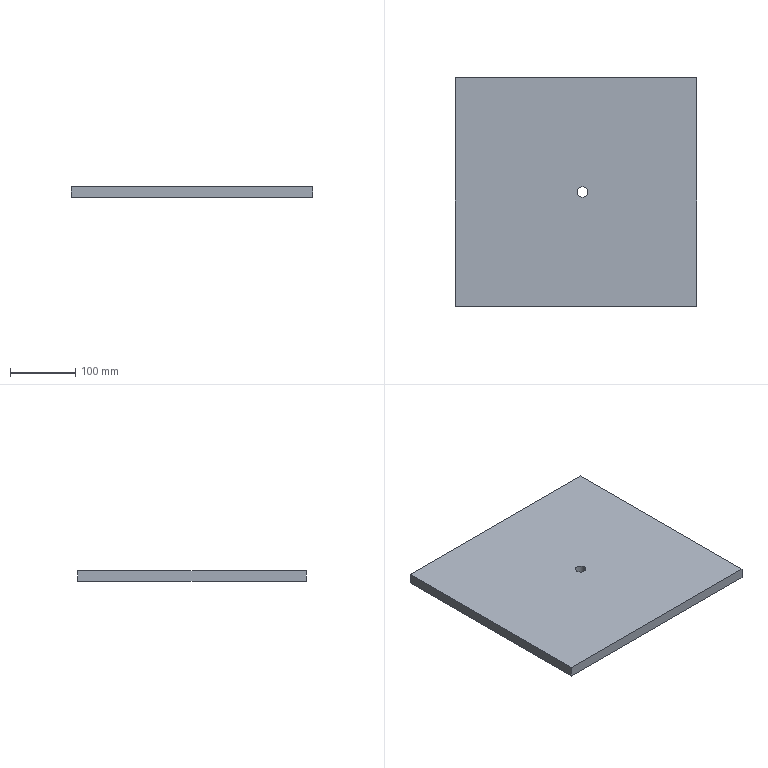Part | SolidWorks | features BaseBody 1 | 1 solid | 8 faces | box 370 x 350 x 16 mm | volume 2068783 mm3 | plane 6 | cylinder 2 | commonest cylinder face diameters 16 x2
STEP:
#1=CARTESIAN_POINT('',(-142.453,1729.544,-1224.));
#2=VERTEX_POINT('',#1);
#3=CARTESIAN_POINT('',(-126.453,1729.544,-1224.));
#4=VERTEX_POINT('',#3);
#5=CARTESIAN_POINT('',(-134.453,1729.544,-1224.));
#6=DIRECTION('',(0.,0.,1.));
#7=DIRECTION('',(1.,0.,0.));
#8=AXIS2_PLACEMENT_3D('',#5,#6,#7);
#9=CIRCLE('',#8,8.);
#10=EDGE_CURVE('',#2,#4,#9,.T.);
#11=ORIENTED_EDGE('',*,*,#10,.F.);
#12=CARTESIAN_POINT('',(-142.453,1729.544,-1208.));
#13=VERTEX_POINT('',#12);
#14=CARTESIAN_POINT('',(-142.453,1729.544,-1246.627));
#15=DIRECTION('',(0.,0.,1.));
#16=VECTOR('',#15,1000.);
#17=LINE('',#14,#16);
#18=EDGE_CURVE('',#2,#13,#17,.T.);
#19=ORIENTED_EDGE('',*,*,#18,.T.);
#20=CARTESIAN_POINT('',(-126.453,1729.544,-1208.));
#21=VERTEX_POINT('',#20);
#22=CARTESIAN_POINT('',(-134.453,1729.544,-1208.));
#23=DIRECTION('',(0.,0.,-1.));
#24=DIRECTION('',(1.,0.,0.));
#25=AXIS2_PLACEMENT_3D('',#22,#23,#24);
#26=CIRCLE('',#25,8.);
#27=EDGE_CURVE('',#21,#13,#26,.T.);
#28=ORIENTED_EDGE('',*,*,#27,.F.);
#29=CARTESIAN_POINT('',(-126.453,1729.544,-1246.627));
#30=DIRECTION('',(0.,0.,1.));
#31=VECTOR('',#30,1000.);
#32=LINE('',#29,#31);
#33=EDGE_CURVE('',#4,#21,#32,.T.);
#34=ORIENTED_EDGE('',*,*,#33,.F.);
#35=EDGE_LOOP('',(#11,#19,#28,#34));
#36=FACE_OUTER_BOUND('',#35,.T.);
#37=CARTESIAN_POINT('',(-134.453,1729.544,-1246.627));
#38=DIRECTION('',(0.,0.,1.));
#39=DIRECTION('',(1.,0.,0.));
#40=AXIS2_PLACEMENT_3D('',#37,#38,#39);
#41=CYLINDRICAL_SURFACE('',#40,8.);
#42=ADVANCED_FACE('',(#36),#41,.F.);
#43=ORIENTED_EDGE('',*,*,#27,.T.);
#44=CARTESIAN_POINT('',(-134.453,1729.544,-1208.));
#45=DIRECTION('',(0.,0.,-1.));
#46=DIRECTION('',(1.,0.,0.));
#47=AXIS2_PLACEMENT_3D('',#44,#45,#46);
#48=CIRCLE('',#47,8.);
#49=EDGE_CURVE('',#13,#21,#48,.T.);
#50=ORIENTED_EDGE('',*,*,#49,.T.);
#51=EDGE_LOOP('',(#43,#50));
#52=FACE_BOUND('',#51,.T.);
#53=CARTESIAN_POINT('',(40.547,1554.544,-1208.));
#54=VERTEX_POINT('',#53);
#55=CARTESIAN_POINT('',(40.547,1904.544,-1208.));
#56=VERTEX_POINT('',#55);
#57=CARTESIAN_POINT('',(40.547,1904.544,-1208.));
#58=DIRECTION('',(0.,1.,0.));
#59=VECTOR('',#58,1000.);
#60=LINE('',#57,#59);
#61=EDGE_CURVE('',#54,#56,#60,.T.);
#62=ORIENTED_EDGE('',*,*,#61,.T.);
#63=CARTESIAN_POINT('',(-329.453,1904.544,-1208.));
#64=VERTEX_POINT('',#63);
#65=CARTESIAN_POINT('',(40.547,1904.544,-1208.));
#66=DIRECTION('',(-1.,0.,0.));
#67=VECTOR('',#66,1000.);
#68=LINE('',#65,#67);
#69=EDGE_CURVE('',#56,#64,#68,.T.);
#70=ORIENTED_EDGE('',*,*,#69,.T.);
#71=CARTESIAN_POINT('',(-329.453,1554.544,-1208.));
#72=VERTEX_POINT('',#71);
#73=CARTESIAN_POINT('',(-329.453,1904.544,-1208.));
#74=DIRECTION('',(0.,-1.,0.));
#75=VECTOR('',#74,1000.);
#76=LINE('',#73,#75);
#77=EDGE_CURVE('',#64,#72,#76,.T.);
#78=ORIENTED_EDGE('',*,*,#77,.T.);
#79=CARTESIAN_POINT('',(40.547,1554.544,-1208.));
#80=DIRECTION('',(1.,0.,0.));
#81=VECTOR('',#80,1000.);
#82=LINE('',#79,#81);
#83=EDGE_CURVE('',#72,#54,#82,.T.);
#84=ORIENTED_EDGE('',*,*,#83,.T.);
#85=EDGE_LOOP('',(#62,#70,#78,#84));
#86=FACE_OUTER_BOUND('',#85,.T.);
#87=CARTESIAN_POINT('',(40.547,1904.544,-1208.));
#88=DIRECTION('',(0.,0.,1.));
#89=DIRECTION('',(1.,0.,0.));
#90=AXIS2_PLACEMENT_3D('',#87,#88,#89);
#91=PLANE('',#90);
#92=ADVANCED_FACE('',(#52,#86),#91,.T.);
#93=ORIENTED_EDGE('',*,*,#18,.F.);
#94=CARTESIAN_POINT('',(-134.453,1729.544,-1224.));
#95=DIRECTION('',(0.,0.,1.));
#96=DIRECTION('',(1.,0.,0.));
#97=AXIS2_PLACEMENT_3D('',#94,#95,#96);
#98=CIRCLE('',#97,8.);
#99=EDGE_CURVE('',#4,#2,#98,.T.);
#100=ORIENTED_EDGE('',*,*,#99,.F.);
#101=ORIENTED_EDGE('',*,*,#33,.T.);
#102=ORIENTED_EDGE('',*,*,#49,.F.);
#103=EDGE_LOOP('',(#93,#100,#101,#102));
#104=FACE_OUTER_BOUND('',#103,.T.);
#105=CARTESIAN_POINT('',(-134.453,1729.544,-1246.627));
#106=DIRECTION('',(0.,0.,1.));
#107=DIRECTION('',(1.,0.,0.));
#108=AXIS2_PLACEMENT_3D('',#105,#106,#107);
#109=CYLINDRICAL_SURFACE('',#108,8.);
#110=ADVANCED_FACE('',(#104),#109,.F.);
#111=ORIENTED_EDGE('',*,*,#69,.F.);
#112=CARTESIAN_POINT('',(40.547,1904.544,-1224.));
#113=VERTEX_POINT('',#112);
#114=CARTESIAN_POINT('',(40.547,1904.544,-1208.));
#115=DIRECTION('',(0.,0.,1.));
#116=VECTOR('',#115,1000.);
#117=LINE('',#114,#116);
#118=EDGE_CURVE('',#113,#56,#117,.T.);
#119=ORIENTED_EDGE('',*,*,#118,.F.);
#120=CARTESIAN_POINT('',(-329.453,1904.544,-1224.));
#121=VERTEX_POINT('',#120);
#122=CARTESIAN_POINT('',(-309.453,1904.544,-1224.));
#123=DIRECTION('',(1.,0.,0.));
#124=VECTOR('',#123,1000.);
#125=LINE('',#122,#124);
#126=EDGE_CURVE('',#121,#113,#125,.T.);
#127=ORIENTED_EDGE('',*,*,#126,.F.);
#128=CARTESIAN_POINT('',(-329.453,1904.544,-1208.));
#129=DIRECTION('',(0.,0.,-1.));
#130=VECTOR('',#129,1000.);
#131=LINE('',#128,#130);
#132=EDGE_CURVE('',#64,#121,#131,.T.);
#133=ORIENTED_EDGE('',*,*,#132,.F.);
#134=EDGE_LOOP('',(#111,#119,#127,#133));
#135=FACE_OUTER_BOUND('',#134,.T.);
#136=CARTESIAN_POINT('',(-309.453,1904.544,-1208.));
#137=DIRECTION('',(0.,-1.,0.));
#138=DIRECTION('',(0.,0.,-1.));
#139=AXIS2_PLACEMENT_3D('',#136,#137,#138);
#140=PLANE('',#139);
#141=ADVANCED_FACE('',(#135),#140,.F.);
#142=ORIENTED_EDGE('',*,*,#61,.F.);
#143=CARTESIAN_POINT('',(40.547,1554.544,-1224.));
#144=VERTEX_POINT('',#143);
#145=CARTESIAN_POINT('',(40.547,1554.544,-1208.));
#146=DIRECTION('',(0.,0.,1.));
#147=VECTOR('',#146,1000.);
#148=LINE('',#145,#147);
#149=EDGE_CURVE('',#144,#54,#148,.T.);
#150=ORIENTED_EDGE('',*,*,#149,.F.);
#151=CARTESIAN_POINT('',(40.547,1554.544,-1224.));
#152=DIRECTION('',(0.,-1.,0.));
#153=VECTOR('',#152,1000.);
#154=LINE('',#151,#153);
#155=EDGE_CURVE('',#113,#144,#154,.T.);
#156=ORIENTED_EDGE('',*,*,#155,.F.);
#157=ORIENTED_EDGE('',*,*,#118,.T.);
#158=EDGE_LOOP('',(#142,#150,#156,#157));
#159=FACE_OUTER_BOUND('',#158,.T.);
#160=CARTESIAN_POINT('',(40.547,1554.544,-1208.));
#161=DIRECTION('',(-1.,0.,0.));
#162=DIRECTION('',(0.,0.,1.));
#163=AXIS2_PLACEMENT_3D('',#160,#161,#162);
#164=PLANE('',#163);
#165=ADVANCED_FACE('',(#159),#164,.F.);
#166=ORIENTED_EDGE('',*,*,#83,.F.);
#167=CARTESIAN_POINT('',(-329.453,1554.544,-1224.));
#168=VERTEX_POINT('',#167);
#169=CARTESIAN_POINT('',(-329.453,1554.544,-1208.));
#170=DIRECTION('',(0.,0.,1.));
#171=VECTOR('',#170,1000.);
#172=LINE('',#169,#171);
#173=EDGE_CURVE('',#168,#72,#172,.T.);
#174=ORIENTED_EDGE('',*,*,#173,.F.);
#175=CARTESIAN_POINT('',(-29.453,1554.544,-1224.));
#176=DIRECTION('',(-1.,0.,0.));
#177=VECTOR('',#176,1000.);
#178=LINE('',#175,#177);
#179=EDGE_CURVE('',#144,#168,#178,.T.);
#180=ORIENTED_EDGE('',*,*,#179,.F.);
#181=ORIENTED_EDGE('',*,*,#149,.T.);
#182=EDGE_LOOP('',(#166,#174,#180,#181));
#183=FACE_OUTER_BOUND('',#182,.T.);
#184=CARTESIAN_POINT('',(-29.453,1554.544,-1208.));
#185=DIRECTION('',(0.,1.,0.));
#186=DIRECTION('',(0.,0.,1.));
#187=AXIS2_PLACEMENT_3D('',#184,#185,#186);
#188=PLANE('',#187);
#189=ADVANCED_FACE('',(#183),#188,.F.);
#190=ORIENTED_EDGE('',*,*,#77,.F.);
#191=ORIENTED_EDGE('',*,*,#132,.T.);
#192=CARTESIAN_POINT('',(-329.453,1554.544,-1224.));
#193=DIRECTION('',(0.,1.,0.));
#194=VECTOR('',#193,1000.);
#195=LINE('',#192,#194);
#196=EDGE_CURVE('',#168,#121,#195,.T.);
#197=ORIENTED_EDGE('',*,*,#196,.F.);
#198=ORIENTED_EDGE('',*,*,#173,.T.);
#199=EDGE_LOOP('',(#190,#191,#197,#198));
#200=FACE_OUTER_BOUND('',#199,.T.);
#201=CARTESIAN_POINT('',(-329.453,1554.544,-1208.));
#202=DIRECTION('',(1.,0.,0.));
#203=DIRECTION('',(0.,0.,-1.));
#204=AXIS2_PLACEMENT_3D('',#201,#202,#203);
#205=PLANE('',#204);
#206=ADVANCED_FACE('',(#200),#205,.F.);
#207=ORIENTED_EDGE('',*,*,#99,.T.);
#208=ORIENTED_EDGE('',*,*,#10,.T.);
#209=EDGE_LOOP('',(#207,#208));
#210=FACE_BOUND('',#209,.T.);
#211=ORIENTED_EDGE('',*,*,#179,.T.);
#212=ORIENTED_EDGE('',*,*,#196,.T.);
#213=ORIENTED_EDGE('',*,*,#126,.T.);
#214=ORIENTED_EDGE('',*,*,#155,.T.);
#215=EDGE_LOOP('',(#211,#212,#213,#214));
#216=FACE_OUTER_BOUND('',#215,.T.);
#217=CARTESIAN_POINT('',(40.547,1904.544,-1224.));
#218=DIRECTION('',(0.,0.,1.));
#219=DIRECTION('',(1.,0.,0.));
#220=AXIS2_PLACEMENT_3D('',#217,#218,#219);
#221=PLANE('',#220);
#222=ADVANCED_FACE('',(#210,#216),#221,.F.);
#223=CLOSED_SHELL('',(#42,#92,#110,#141,#165,#189,#206,#222));
#224=MANIFOLD_SOLID_BREP('',#223);
#225=CARTESIAN_POINT('',(0.,0.,0.));
#226=DIRECTION('',(0.,0.,1.));
#227=DIRECTION('',(1.,0.,0.));
#228=AXIS2_PLACEMENT_3D('',#225,#226,#227);
#229=(LENGTH_UNIT()NAMED_UNIT(*)SI_UNIT(.MILLI.,.METRE.));
#230=UNCERTAINTY_MEASURE_WITH_UNIT(LENGTH_MEASURE(0.00001),#229,'','');
#231=(NAMED_UNIT(*)PLANE_ANGLE_UNIT()SI_UNIT($,.RADIAN.));
#232=(NAMED_UNIT(*)SI_UNIT($,.STERADIAN.)SOLID_ANGLE_UNIT());
#233=(GEOMETRIC_REPRESENTATION_CONTEXT(3)GLOBAL_UNCERTAINTY_ASSIGNED_CONTEXT((#230))GLOBAL_UNIT_ASSIGNED_CONTEXT((#229,#231,#232))REPRESENTATION_CONTEXT('',''));
#234=ADVANCED_BREP_SHAPE_REPRESENTATION('',(#224,#228),#233);